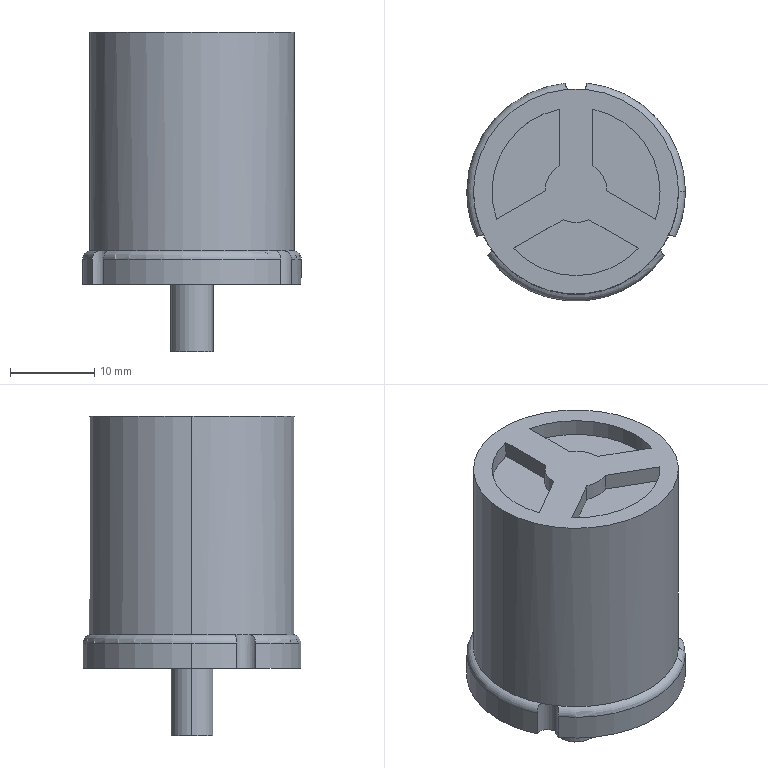Part | SolidWorks | features ICE 6, Fillet 2, Extrusion 1 | 1 solid | 53 faces | box 26 x 25.935 x 38 mm | volume 13857 mm3 | cylinder 25 | plane 20 | torus 8 | commonest cylinder face diameters 3 x6 2.6 x4 20 x4 26 x4 7.378 x3 5 x2